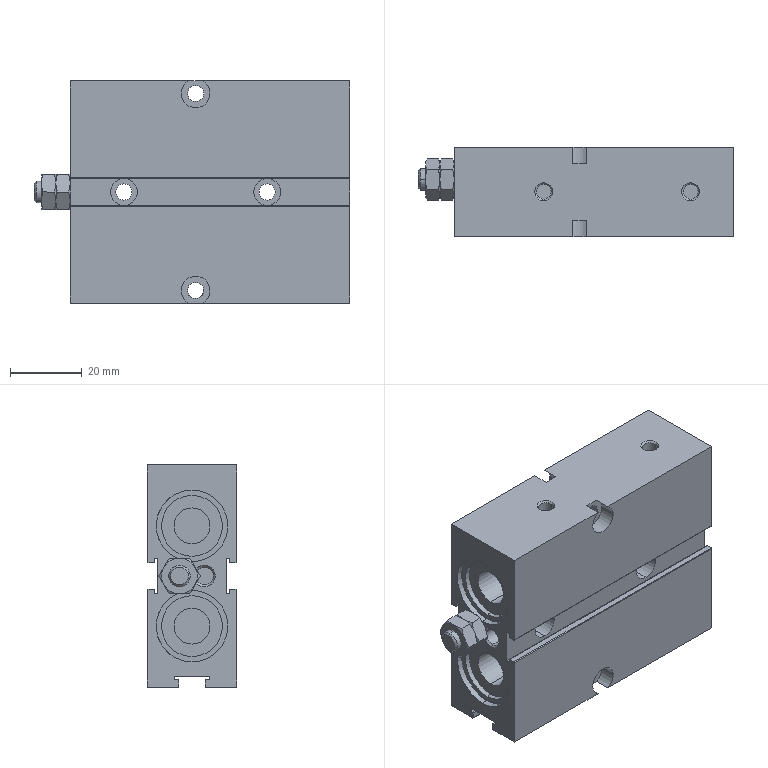Part | SolidWorks | features BaseBody 1 | 1 solid | 189 faces | box 88 x 25 x 62 mm | volume 82875 mm3 | cylinder 82 | plane 75 | cone 32 | commonest cylinder face diameters 0.4 x30 20 x12 4.5 x8 7.5 x8 17 x8 4.134 x4